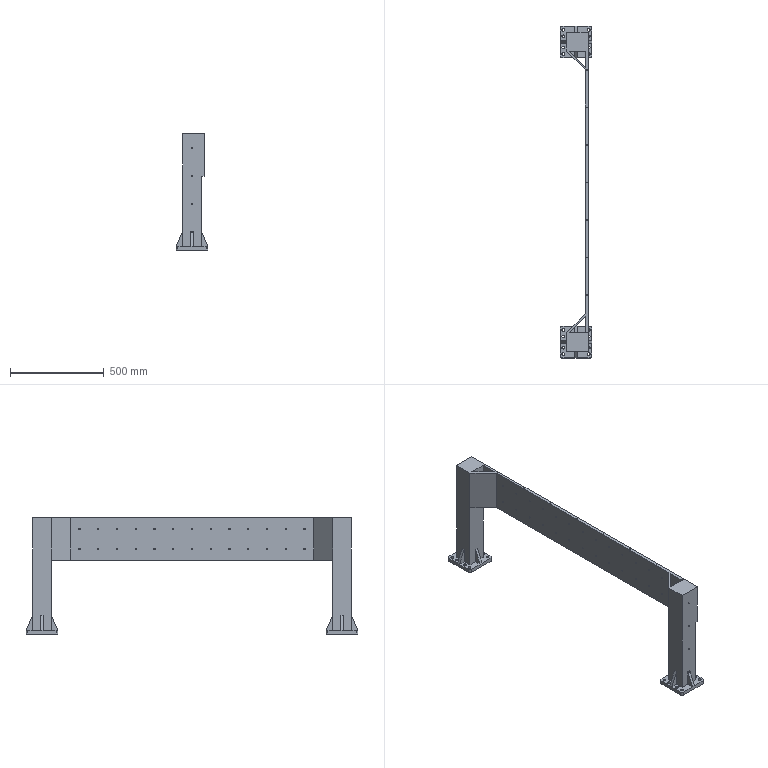Part | STEP file | 1 solid | 263 faces | box 170 x 1770 x 620 mm | volume 19562829 mm3 | cylinder 150 | plane 67 | cone 46 | commonest cylinder face diameters 6.8 x68 15 x32 4.2 x30 10 x12 20 x8